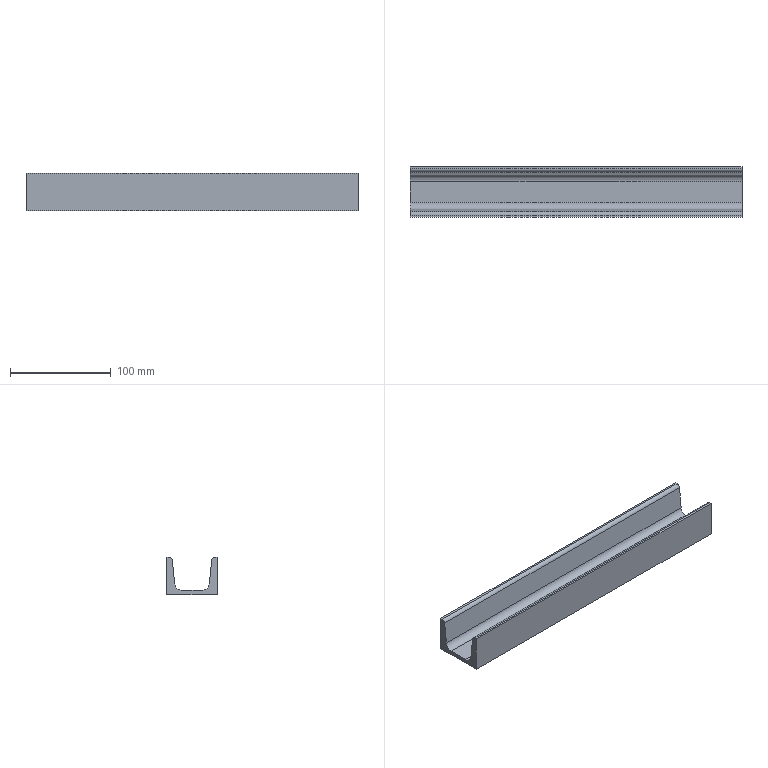Part | STEP file | HESS-408-70-15W-W-39-5# channel 1_default_machined_ | 1 solid | 14 faces | box 330 x 50 x 37 mm | volume 223683 mm3 | plane 10 | cylinder 4 | commonest cylinder face diameters 7 x2 14 x2
STEP:
#1=CARTESIAN_POINT('',(0.,0.,0.));
#2=DIRECTION('',(0.,0.,1.));
#3=DIRECTION('',(1.,0.,0.));
#4=AXIS2_PLACEMENT_3D('',#1,#2,#3);
#5=CARTESIAN_POINT('',(330.,0.,0.));
#6=VERTEX_POINT('',#5);
#7=CARTESIAN_POINT('',(0.,0.,0.));
#8=VERTEX_POINT('',#7);
#9=CARTESIAN_POINT('',(330.,0.,0.));
#10=DIRECTION('',(-1.,0.,0.));
#11=VECTOR('',#10,1.);
#12=LINE('',#9,#11);
#13=CARTESIAN_POINT('',(330.,0.,0.));
#14=DIRECTION('',(0.,0.,1.));
#15=DIRECTION('',(0.,-1.,0.));
#16=AXIS2_PLACEMENT_3D('',#13,#14,#15);
#17=PLANE('',#16);
#18=CARTESIAN_POINT('',(0.,0.));
#19=DIRECTION('',(0.,-1.));
#20=VECTOR('',#19,1.);
#21=LINE('',#18,#20);
#22=(GEOMETRIC_REPRESENTATION_CONTEXT(2)PARAMETRIC_REPRESENTATION_CONTEXT()REPRESENTATION_CONTEXT('',''));
#23=DEFINITIONAL_REPRESENTATION('',(#21),#22);
#24=PCURVE('',#17,#23);
#25=CARTESIAN_POINT('',(330.,0.,0.));
#26=DIRECTION('',(0.,-1.,0.));
#27=DIRECTION('',(0.,0.,-1.));
#28=AXIS2_PLACEMENT_3D('',#25,#26,#27);
#29=PLANE('',#28);
#30=CARTESIAN_POINT('',(0.,0.));
#31=DIRECTION('',(0.,-1.));
#32=VECTOR('',#31,1.);
#33=LINE('',#30,#32);
#34=(GEOMETRIC_REPRESENTATION_CONTEXT(2)PARAMETRIC_REPRESENTATION_CONTEXT()REPRESENTATION_CONTEXT('',''));
#35=DEFINITIONAL_REPRESENTATION('',(#33),#34);
#36=PCURVE('',#29,#35);
#37=SURFACE_CURVE('',#12,(#24,#36),.PCURVE_S1.);
#38=EDGE_CURVE('',#6,#8,#37,.T.);
#39=ORIENTED_EDGE('',*,*,#38,.F.);
#40=CARTESIAN_POINT('',(330.,-50.,0.));
#41=VERTEX_POINT('',#40);
#42=CARTESIAN_POINT('',(330.,0.,0.));
#43=DIRECTION('',(0.,1.,0.));
#44=VECTOR('',#43,1.);
#45=LINE('',#42,#44);
#46=CARTESIAN_POINT('',(0.,0.));
#47=DIRECTION('',(-1.,0.));
#48=VECTOR('',#47,1.);
#49=LINE('',#46,#48);
#50=(GEOMETRIC_REPRESENTATION_CONTEXT(2)PARAMETRIC_REPRESENTATION_CONTEXT()REPRESENTATION_CONTEXT('',''));
#51=DEFINITIONAL_REPRESENTATION('',(#49),#50);
#52=PCURVE('',#17,#51);
#53=CARTESIAN_POINT('',(330.,-48.017,33.5));
#54=DIRECTION('',(1.,0.,0.));
#55=DIRECTION('',(0.,1.,0.));
#56=AXIS2_PLACEMENT_3D('',#53,#54,#55);
#57=PLANE('',#56);
#58=CARTESIAN_POINT('',(48.017,-33.5));
#59=DIRECTION('',(1.,0.));
#60=VECTOR('',#59,1.);
#61=LINE('',#58,#60);
#62=(GEOMETRIC_REPRESENTATION_CONTEXT(2)PARAMETRIC_REPRESENTATION_CONTEXT()REPRESENTATION_CONTEXT('',''));
#63=DEFINITIONAL_REPRESENTATION('',(#61),#62);
#64=PCURVE('',#57,#63);
#65=SURFACE_CURVE('',#45,(#52,#64),.PCURVE_S1.);
#66=EDGE_CURVE('',#41,#6,#65,.T.);
#67=ORIENTED_EDGE('',*,*,#66,.F.);
#68=CARTESIAN_POINT('',(0.,-50.,0.));
#69=VERTEX_POINT('',#68);
#70=CARTESIAN_POINT('',(330.,-50.,0.));
#71=DIRECTION('',(1.,0.,0.));
#72=VECTOR('',#71,1.);
#73=LINE('',#70,#72);
#74=CARTESIAN_POINT('',(50.,0.));
#75=DIRECTION('',(0.,1.));
#76=VECTOR('',#75,1.);
#77=LINE('',#74,#76);
#78=(GEOMETRIC_REPRESENTATION_CONTEXT(2)PARAMETRIC_REPRESENTATION_CONTEXT()REPRESENTATION_CONTEXT('',''));
#79=DEFINITIONAL_REPRESENTATION('',(#77),#78);
#80=PCURVE('',#17,#79);
#81=CARTESIAN_POINT('',(330.,-50.,0.));
#82=DIRECTION('',(0.,1.,0.));
#83=DIRECTION('',(0.,0.,1.));
#84=AXIS2_PLACEMENT_3D('',#81,#82,#83);
#85=PLANE('',#84);
#86=CARTESIAN_POINT('',(0.,0.));
#87=DIRECTION('',(0.,1.));
#88=VECTOR('',#87,1.);
#89=LINE('',#86,#88);
#90=(GEOMETRIC_REPRESENTATION_CONTEXT(2)PARAMETRIC_REPRESENTATION_CONTEXT()REPRESENTATION_CONTEXT('',''));
#91=DEFINITIONAL_REPRESENTATION('',(#89),#90);
#92=PCURVE('',#85,#91);
#93=SURFACE_CURVE('',#73,(#80,#92),.PCURVE_S1.);
#94=EDGE_CURVE('',#69,#41,#93,.T.);
#95=ORIENTED_EDGE('',*,*,#94,.F.);
#96=CARTESIAN_POINT('',(0.,0.,0.));
#97=DIRECTION('',(0.,-1.,0.));
#98=VECTOR('',#97,1.);
#99=LINE('',#96,#98);
#100=CARTESIAN_POINT('',(0.,-330.));
#101=DIRECTION('',(1.,0.));
#102=VECTOR('',#101,1.);
#103=LINE('',#100,#102);
#104=(GEOMETRIC_REPRESENTATION_CONTEXT(2)PARAMETRIC_REPRESENTATION_CONTEXT()REPRESENTATION_CONTEXT('',''));
#105=DEFINITIONAL_REPRESENTATION('',(#103),#104);
#106=PCURVE('',#17,#105);
#107=CARTESIAN_POINT('',(0.,-48.017,33.5));
#108=DIRECTION('',(1.,0.,0.));
#109=DIRECTION('',(0.,1.,0.));
#110=AXIS2_PLACEMENT_3D('',#107,#108,#109);
#111=PLANE('',#110);
#112=CARTESIAN_POINT('',(48.017,-33.5));
#113=DIRECTION('',(-1.,0.));
#114=VECTOR('',#113,1.);
#115=LINE('',#112,#114);
#116=(GEOMETRIC_REPRESENTATION_CONTEXT(2)PARAMETRIC_REPRESENTATION_CONTEXT()REPRESENTATION_CONTEXT('',''));
#117=DEFINITIONAL_REPRESENTATION('',(#115),#116);
#118=PCURVE('',#111,#117);
#119=SURFACE_CURVE('',#99,(#106,#118),.PCURVE_S1.);
#120=EDGE_CURVE('',#8,#69,#119,.T.);
#121=ORIENTED_EDGE('',*,*,#120,.F.);
#122=EDGE_LOOP('',(#39,#67,#95,#121));
#123=FACE_BOUND('',#122,.T.);
#124=ADVANCED_FACE('',(#123),#17,.F.);
#125=CARTESIAN_POINT('',(0.,-48.017,37.));
#126=VERTEX_POINT('',#125);
#127=CARTESIAN_POINT('',(0.,-50.,37.));
#128=VERTEX_POINT('',#127);
#129=CARTESIAN_POINT('',(0.,-48.017,37.));
#130=DIRECTION('',(0.,-1.,0.));
#131=VECTOR('',#130,1.);
#132=LINE('',#129,#131);
#133=CARTESIAN_POINT('',(0.,3.5));
#134=DIRECTION('',(-1.,0.));
#135=VECTOR('',#134,1.);
#136=LINE('',#133,#135);
#137=(GEOMETRIC_REPRESENTATION_CONTEXT(2)PARAMETRIC_REPRESENTATION_CONTEXT()REPRESENTATION_CONTEXT('',''));
#138=DEFINITIONAL_REPRESENTATION('',(#136),#137);
#139=PCURVE('',#111,#138);
#140=CARTESIAN_POINT('',(330.,-48.017,37.));
#141=DIRECTION('',(0.,0.,-1.));
#142=DIRECTION('',(0.,1.,0.));
#143=AXIS2_PLACEMENT_3D('',#140,#141,#142);
#144=PLANE('',#143);
#145=CARTESIAN_POINT('',(0.,-330.));
#146=DIRECTION('',(-1.,0.));
#147=VECTOR('',#146,1.);
#148=LINE('',#145,#147);
#149=(GEOMETRIC_REPRESENTATION_CONTEXT(2)PARAMETRIC_REPRESENTATION_CONTEXT()REPRESENTATION_CONTEXT('',''));
#150=DEFINITIONAL_REPRESENTATION('',(#148),#149);
#151=PCURVE('',#144,#150);
#152=SURFACE_CURVE('',#132,(#139,#151),.PCURVE_S1.);
#153=EDGE_CURVE('',#126,#128,#152,.T.);
#154=ORIENTED_EDGE('',*,*,#153,.F.);
#155=CARTESIAN_POINT('',(0.,-44.535,33.848));
#156=VERTEX_POINT('',#155);
#157=CARTESIAN_POINT('',(0.,-48.017,33.5));
#158=DIRECTION('',(1.,0.,0.));
#159=DIRECTION('',(0.,-1.,0.));
#160=AXIS2_PLACEMENT_3D('',#157,#158,#159);
#161=CIRCLE('',#160,3.5);
#162=CARTESIAN_POINT('',(0.,0.));
#163=DIRECTION('',(-1.,0.));
#164=AXIS2_PLACEMENT_2D('',#162,#163);
#165=CIRCLE('',#164,3.5);
#166=(GEOMETRIC_REPRESENTATION_CONTEXT(2)PARAMETRIC_REPRESENTATION_CONTEXT()REPRESENTATION_CONTEXT('',''));
#167=DEFINITIONAL_REPRESENTATION('',(#165),#166);
#168=PCURVE('',#111,#167);
#169=CARTESIAN_POINT('',(330.,-48.017,33.5));
#170=DIRECTION('',(-1.,0.,0.));
#171=DIRECTION('',(0.,-1.,0.));
#172=AXIS2_PLACEMENT_3D('',#169,#170,#171);
#173=CYLINDRICAL_SURFACE('',#172,3.5);
#174=CARTESIAN_POINT('',(6.283,330.));
#175=DIRECTION('',(-1.,0.));
#176=VECTOR('',#175,1.);
#177=LINE('',#174,#176);
#178=(GEOMETRIC_REPRESENTATION_CONTEXT(2)PARAMETRIC_REPRESENTATION_CONTEXT()REPRESENTATION_CONTEXT('',''));
#179=DEFINITIONAL_REPRESENTATION('',(#177),#178);
#180=PCURVE('',#173,#179);
#181=SURFACE_CURVE('',#161,(#168,#180),.PCURVE_S1.);
#182=EDGE_CURVE('',#156,#126,#181,.T.);
#183=ORIENTED_EDGE('',*,*,#182,.F.);
#184=CARTESIAN_POINT('',(0.,-42.23,10.803));
#185=VERTEX_POINT('',#184);
#186=CARTESIAN_POINT('',(0.,-42.23,10.803));
#187=DIRECTION('',(0.,-0.0995,0.995));
#188=VECTOR('',#187,1.);
#189=LINE('',#186,#188);
#190=CARTESIAN_POINT('',(5.787,-22.697));
#191=DIRECTION('',(-0.0995,0.995));
#192=VECTOR('',#191,1.);
#193=LINE('',#190,#192);
#194=(GEOMETRIC_REPRESENTATION_CONTEXT(2)PARAMETRIC_REPRESENTATION_CONTEXT()REPRESENTATION_CONTEXT('',''));
#195=DEFINITIONAL_REPRESENTATION('',(#193),#194);
#196=PCURVE('',#111,#195);
#197=CARTESIAN_POINT('',(330.,-42.23,10.803));
#198=DIRECTION('',(0.,-0.995,-0.0995));
#199=DIRECTION('',(0.,0.0995,-0.995));
#200=AXIS2_PLACEMENT_3D('',#197,#198,#199);
#201=PLANE('',#200);
#202=CARTESIAN_POINT('',(0.,-330.));
#203=DIRECTION('',(-1.,0.));
#204=VECTOR('',#203,1.);
#205=LINE('',#202,#204);
#206=(GEOMETRIC_REPRESENTATION_CONTEXT(2)PARAMETRIC_REPRESENTATION_CONTEXT()REPRESENTATION_CONTEXT('',''));
#207=DEFINITIONAL_REPRESENTATION('',(#205),#206);
#208=PCURVE('',#201,#207);
#209=SURFACE_CURVE('',#189,(#196,#208),.PCURVE_S1.);
#210=EDGE_CURVE('',#185,#156,#209,.T.);
#211=ORIENTED_EDGE('',*,*,#210,.F.);
#212=CARTESIAN_POINT('',(0.,-35.265,4.5));
#213=VERTEX_POINT('',#212);
#214=CARTESIAN_POINT('',(0.,-35.265,11.5));
#215=DIRECTION('',(-1.,0.,0.));
#216=DIRECTION('',(0.,-1.,0.));
#217=AXIS2_PLACEMENT_3D('',#214,#215,#216);
#218=CIRCLE('',#217,7.);
#219=CARTESIAN_POINT('',(5.752,-22.));
#220=CARTESIAN_POINT('',(5.752,-9.876));
#221=CARTESIAN_POINT('',(16.252,-15.938));
#222=CARTESIAN_POINT('',(26.752,-22.));
#223=CARTESIAN_POINT('',(16.252,-28.062));
#224=CARTESIAN_POINT('',(5.752,-34.124));
#225=CARTESIAN_POINT('',(5.752,-22.));
#226=(BOUNDED_CURVE()B_SPLINE_CURVE(2,(#219,#220,#221,#222,#223,#224,#225),.UNSPECIFIED.,.T.,.F.)B_SPLINE_CURVE_WITH_KNOTS((1,2,2,2,2,1),(-2.094,0.,2.094,4.189,6.283,8.378),.UNSPECIFIED.)CURVE()GEOMETRIC_REPRESENTATION_ITEM()RATIONAL_B_SPLINE_CURVE((1.,0.5,1.,0.5,1.,0.5,1.))REPRESENTATION_ITEM(''));
#227=(GEOMETRIC_REPRESENTATION_CONTEXT(2)PARAMETRIC_REPRESENTATION_CONTEXT()REPRESENTATION_CONTEXT('',''));
#228=DEFINITIONAL_REPRESENTATION('',(#226),#227);
#229=PCURVE('',#111,#228);
#230=CARTESIAN_POINT('',(330.,-35.265,11.5));
#231=DIRECTION('',(-1.,0.,0.));
#232=DIRECTION('',(0.,-1.,0.));
#233=AXIS2_PLACEMENT_3D('',#230,#231,#232);
#234=CYLINDRICAL_SURFACE('',#233,7.);
#235=CARTESIAN_POINT('',(0.,330.));
#236=DIRECTION('',(1.,0.));
#237=VECTOR('',#236,1.);
#238=LINE('',#235,#237);
#239=(GEOMETRIC_REPRESENTATION_CONTEXT(2)PARAMETRIC_REPRESENTATION_CONTEXT()REPRESENTATION_CONTEXT('',''));
#240=DEFINITIONAL_REPRESENTATION('',(#238),#239);
#241=PCURVE('',#234,#240);
#242=SURFACE_CURVE('',#218,(#229,#241),.PCURVE_S1.);
#243=EDGE_CURVE('',#213,#185,#242,.T.);
#244=ORIENTED_EDGE('',*,*,#243,.F.);
#245=CARTESIAN_POINT('',(0.,-14.735,4.5));
#246=VERTEX_POINT('',#245);
#247=CARTESIAN_POINT('',(0.,-48.017,4.5));
#248=DIRECTION('',(0.,-1.,0.));
#249=VECTOR('',#248,1.);
#250=LINE('',#247,#249);
#251=CARTESIAN_POINT('',(0.,-29.));
#252=DIRECTION('',(-1.,0.));
#253=VECTOR('',#252,1.);
#254=LINE('',#251,#253);
#255=(GEOMETRIC_REPRESENTATION_CONTEXT(2)PARAMETRIC_REPRESENTATION_CONTEXT()REPRESENTATION_CONTEXT('',''));
#256=DEFINITIONAL_REPRESENTATION('',(#254),#255);
#257=PCURVE('',#111,#256);
#258=CARTESIAN_POINT('',(330.,-35.265,4.5));
#259=DIRECTION('',(0.,0.,-1.));
#260=DIRECTION('',(0.,1.,0.));
#261=AXIS2_PLACEMENT_3D('',#258,#259,#260);
#262=PLANE('',#261);
#263=CARTESIAN_POINT('',(-12.752,-330.));
#264=DIRECTION('',(-1.,0.));
#265=VECTOR('',#264,1.);
#266=LINE('',#263,#265);
#267=(GEOMETRIC_REPRESENTATION_CONTEXT(2)PARAMETRIC_REPRESENTATION_CONTEXT()REPRESENTATION_CONTEXT('',''));
#268=DEFINITIONAL_REPRESENTATION('',(#266),#267);
#269=PCURVE('',#262,#268);
#270=SURFACE_CURVE('',#250,(#257,#269),.PCURVE_S1.);
#271=EDGE_CURVE('',#246,#213,#270,.T.);
#272=ORIENTED_EDGE('',*,*,#271,.F.);
#273=CARTESIAN_POINT('',(0.,-7.77,10.803));
#274=VERTEX_POINT('',#273);
#275=CARTESIAN_POINT('',(0.,-14.735,11.5));
#276=DIRECTION('',(-1.,0.,0.));
#277=DIRECTION('',(0.,-1.,0.));
#278=AXIS2_PLACEMENT_3D('',#275,#276,#277);
#279=CIRCLE('',#278,7.);
#280=CARTESIAN_POINT('',(26.283,-22.));
#281=CARTESIAN_POINT('',(26.283,-9.876));
#282=CARTESIAN_POINT('',(36.783,-15.938));
#283=CARTESIAN_POINT('',(47.283,-22.));
#284=CARTESIAN_POINT('',(36.783,-28.062));
#285=CARTESIAN_POINT('',(26.283,-34.124));
#286=CARTESIAN_POINT('',(26.283,-22.));
#287=(BOUNDED_CURVE()B_SPLINE_CURVE(2,(#280,#281,#282,#283,#284,#285,#286),.UNSPECIFIED.,.T.,.F.)B_SPLINE_CURVE_WITH_KNOTS((1,2,2,2,2,1),(-2.094,0.,2.094,4.189,6.283,8.378),.UNSPECIFIED.)CURVE()GEOMETRIC_REPRESENTATION_ITEM()RATIONAL_B_SPLINE_CURVE((1.,0.5,1.,0.5,1.,0.5,1.))REPRESENTATION_ITEM(''));
#288=(GEOMETRIC_REPRESENTATION_CONTEXT(2)PARAMETRIC_REPRESENTATION_CONTEXT()REPRESENTATION_CONTEXT('',''));
#289=DEFINITIONAL_REPRESENTATION('',(#287),#288);
#290=PCURVE('',#111,#289);
#291=CARTESIAN_POINT('',(330.,-14.735,11.5));
#292=DIRECTION('',(-1.,0.,0.));
#293=DIRECTION('',(0.,-1.,0.));
#294=AXIS2_PLACEMENT_3D('',#291,#292,#293);
#295=CYLINDRICAL_SURFACE('',#294,7.);
#296=CARTESIAN_POINT('',(0.,330.));
#297=DIRECTION('',(1.,0.));
#298=VECTOR('',#297,1.);
#299=LINE('',#296,#298);
#300=(GEOMETRIC_REPRESENTATION_CONTEXT(2)PARAMETRIC_REPRESENTATION_CONTEXT()REPRESENTATION_CONTEXT('',''));
#301=DEFINITIONAL_REPRESENTATION('',(#299),#300);
#302=PCURVE('',#295,#301);
#303=SURFACE_CURVE('',#279,(#290,#302),.PCURVE_S1.);
#304=EDGE_CURVE('',#274,#246,#303,.T.);
#305=ORIENTED_EDGE('',*,*,#304,.F.);
#306=CARTESIAN_POINT('',(0.,-5.465,33.848));
#307=VERTEX_POINT('',#306);
#308=CARTESIAN_POINT('',(0.,-5.465,33.848));
#309=DIRECTION('',(0.,-0.0995,-0.995));
#310=VECTOR('',#309,1.);
#311=LINE('',#308,#310);
#312=CARTESIAN_POINT('',(42.552,0.3483));
#313=DIRECTION('',(-0.0995,-0.995));
#314=VECTOR('',#313,1.);
#315=LINE('',#312,#314);
#316=(GEOMETRIC_REPRESENTATION_CONTEXT(2)PARAMETRIC_REPRESENTATION_CONTEXT()REPRESENTATION_CONTEXT('',''));
#317=DEFINITIONAL_REPRESENTATION('',(#315),#316);
#318=PCURVE('',#111,#317);
#319=CARTESIAN_POINT('',(330.,-7.77,10.803));
#320=DIRECTION('',(0.,0.995,-0.0995));
#321=DIRECTION('',(0.,0.0995,0.995));
#322=AXIS2_PLACEMENT_3D('',#319,#320,#321);
#323=PLANE('',#322);
#324=CARTESIAN_POINT('',(23.16,-330.));
#325=DIRECTION('',(-1.,0.));
#326=VECTOR('',#325,1.);
#327=LINE('',#324,#326);
#328=(GEOMETRIC_REPRESENTATION_CONTEXT(2)PARAMETRIC_REPRESENTATION_CONTEXT()REPRESENTATION_CONTEXT('',''));
#329=DEFINITIONAL_REPRESENTATION('',(#327),#328);
#330=PCURVE('',#323,#329);
#331=SURFACE_CURVE('',#311,(#318,#330),.PCURVE_S1.);
#332=EDGE_CURVE('',#307,#274,#331,.T.);
#333=ORIENTED_EDGE('',*,*,#332,.F.);
#334=CARTESIAN_POINT('',(0.,-1.983,37.));
#335=VERTEX_POINT('',#334);
#336=CARTESIAN_POINT('',(0.,-1.983,33.5));
#337=DIRECTION('',(1.,0.,0.));
#338=DIRECTION('',(0.,-1.,0.));
#339=AXIS2_PLACEMENT_3D('',#336,#337,#338);
#340=CIRCLE('',#339,3.5);
#341=CARTESIAN_POINT('',(46.035,0.));
#342=DIRECTION('',(-1.,0.));
#343=AXIS2_PLACEMENT_2D('',#341,#342);
#344=CIRCLE('',#343,3.5);
#345=(GEOMETRIC_REPRESENTATION_CONTEXT(2)PARAMETRIC_REPRESENTATION_CONTEXT()REPRESENTATION_CONTEXT('',''));
#346=DEFINITIONAL_REPRESENTATION('',(#344),#345);
#347=PCURVE('',#111,#346);
#348=CARTESIAN_POINT('',(330.,-1.983,33.5));
#349=DIRECTION('',(-1.,0.,0.));
#350=DIRECTION('',(0.,-1.,0.));
#351=AXIS2_PLACEMENT_3D('',#348,#349,#350);
#352=CYLINDRICAL_SURFACE('',#351,3.5);
#353=CARTESIAN_POINT('',(6.283,330.));
#354=DIRECTION('',(-1.,0.));
#355=VECTOR('',#354,1.);
#356=LINE('',#353,#355);
#357=(GEOMETRIC_REPRESENTATION_CONTEXT(2)PARAMETRIC_REPRESENTATION_CONTEXT()REPRESENTATION_CONTEXT('',''));
#358=DEFINITIONAL_REPRESENTATION('',(#356),#357);
#359=PCURVE('',#352,#358);
#360=SURFACE_CURVE('',#340,(#347,#359),.PCURVE_S1.);
#361=EDGE_CURVE('',#335,#307,#360,.T.);
#362=ORIENTED_EDGE('',*,*,#361,.F.);
#363=CARTESIAN_POINT('',(0.,0.,37.));
#364=VERTEX_POINT('',#363);
#365=CARTESIAN_POINT('',(0.,-48.017,37.));
#366=DIRECTION('',(0.,-1.,0.));
#367=VECTOR('',#366,1.);
#368=LINE('',#365,#367);
#369=CARTESIAN_POINT('',(0.,3.5));
#370=DIRECTION('',(-1.,0.));
#371=VECTOR('',#370,1.);
#372=LINE('',#369,#371);
#373=(GEOMETRIC_REPRESENTATION_CONTEXT(2)PARAMETRIC_REPRESENTATION_CONTEXT()REPRESENTATION_CONTEXT('',''));
#374=DEFINITIONAL_REPRESENTATION('',(#372),#373);
#375=PCURVE('',#111,#374);
#376=CARTESIAN_POINT('',(330.,-1.983,37.));
#377=DIRECTION('',(0.,0.,-1.));
#378=DIRECTION('',(0.,1.,0.));
#379=AXIS2_PLACEMENT_3D('',#376,#377,#378);
#380=PLANE('',#379);
#381=CARTESIAN_POINT('',(-46.035,-330.));
#382=DIRECTION('',(-1.,0.));
#383=VECTOR('',#382,1.);
#384=LINE('',#381,#383);
#385=(GEOMETRIC_REPRESENTATION_CONTEXT(2)PARAMETRIC_REPRESENTATION_CONTEXT()REPRESENTATION_CONTEXT('',''));
#386=DEFINITIONAL_REPRESENTATION('',(#384),#385);
#387=PCURVE('',#380,#386);
#388=SURFACE_CURVE('',#368,(#375,#387),.PCURVE_S1.);
#389=EDGE_CURVE('',#364,#335,#388,.T.);
#390=ORIENTED_EDGE('',*,*,#389,.F.);
#391=CARTESIAN_POINT('',(0.,0.,33.5));
#392=DIRECTION('',(0.,0.,1.));
#393=VECTOR('',#392,1.);
#394=LINE('',#391,#393);
#395=CARTESIAN_POINT('',(48.017,0.));
#396=DIRECTION('',(0.,1.));
#397=VECTOR('',#396,1.);
#398=LINE('',#395,#397);
#399=(GEOMETRIC_REPRESENTATION_CONTEXT(2)PARAMETRIC_REPRESENTATION_CONTEXT()REPRESENTATION_CONTEXT('',''));
#400=DEFINITIONAL_REPRESENTATION('',(#398),#399);
#401=PCURVE('',#111,#400);
#402=CARTESIAN_POINT('',(-33.5,-330.));
#403=DIRECTION('',(-1.,0.));
#404=VECTOR('',#403,1.);
#405=LINE('',#402,#404);
#406=(GEOMETRIC_REPRESENTATION_CONTEXT(2)PARAMETRIC_REPRESENTATION_CONTEXT()REPRESENTATION_CONTEXT('',''));
#407=DEFINITIONAL_REPRESENTATION('',(#405),#406);
#408=PCURVE('',#29,#407);
#409=SURFACE_CURVE('',#394,(#401,#408),.PCURVE_S1.);
#410=EDGE_CURVE('',#8,#364,#409,.T.);
#411=ORIENTED_EDGE('',*,*,#410,.F.);
#412=ORIENTED_EDGE('',*,*,#120,.T.);
#413=CARTESIAN_POINT('',(0.,-50.,33.5));
#414=DIRECTION('',(0.,0.,-1.));
#415=VECTOR('',#414,1.);
#416=LINE('',#413,#415);
#417=CARTESIAN_POINT('',(-1.983,0.));
#418=DIRECTION('',(0.,-1.));
#419=VECTOR('',#418,1.);
#420=LINE('',#417,#419);
#421=(GEOMETRIC_REPRESENTATION_CONTEXT(2)PARAMETRIC_REPRESENTATION_CONTEXT()REPRESENTATION_CONTEXT('',''));
#422=DEFINITIONAL_REPRESENTATION('',(#420),#421);
#423=PCURVE('',#111,#422);
#424=CARTESIAN_POINT('',(33.5,-330.));
#425=DIRECTION('',(-1.,0.));
#426=VECTOR('',#425,1.);
#427=LINE('',#424,#426);
#428=(GEOMETRIC_REPRESENTATION_CONTEXT(2)PARAMETRIC_REPRESENTATION_CONTEXT()REPRESENTATION_CONTEXT('',''));
#429=DEFINITIONAL_REPRESENTATION('',(#427),#428);
#430=PCURVE('',#85,#429);
#431=SURFACE_CURVE('',#416,(#423,#430),.PCURVE_S1.);
#432=EDGE_CURVE('',#128,#69,#431,.T.);
#433=ORIENTED_EDGE('',*,*,#432,.F.);
#434=EDGE_LOOP('',(#154,#183,#211,#244,#272,#305,#333,#362,#390,#411,#412,#433));
#435=FACE_BOUND('',#434,.T.);
#436=ADVANCED_FACE('',(#435),#111,.F.);
#437=CARTESIAN_POINT('',(330.,0.,37.));
#438=VERTEX_POINT('',#437);
#439=CARTESIAN_POINT('',(330.,0.,37.));
#440=DIRECTION('',(-1.,0.,0.));
#441=VECTOR('',#440,1.);
#442=LINE('',#439,#441);
#443=CARTESIAN_POINT('',(-37.,0.));
#444=DIRECTION('',(0.,-1.));
#445=VECTOR('',#444,1.);
#446=LINE('',#443,#445);
#447=(GEOMETRIC_REPRESENTATION_CONTEXT(2)PARAMETRIC_REPRESENTATION_CONTEXT()REPRESENTATION_CONTEXT('',''));
#448=DEFINITIONAL_REPRESENTATION('',(#446),#447);
#449=PCURVE('',#29,#448);
#450=CARTESIAN_POINT('',(1.983,0.));
#451=DIRECTION('',(0.,-1.));
#452=VECTOR('',#451,1.);
#453=LINE('',#450,#452);
#454=(GEOMETRIC_REPRESENTATION_CONTEXT(2)PARAMETRIC_REPRESENTATION_CONTEXT()REPRESENTATION_CONTEXT('',''));
#455=DEFINITIONAL_REPRESENTATION('',(#453),#454);
#456=PCURVE('',#380,#455);
#457=SURFACE_CURVE('',#442,(#449,#456),.PCURVE_S1.);
#458=EDGE_CURVE('',#438,#364,#457,.T.);
#459=ORIENTED_EDGE('',*,*,#458,.F.);
#460=CARTESIAN_POINT('',(330.,0.,0.));
#461=DIRECTION('',(0.,0.,1.));
#462=VECTOR('',#461,1.);
#463=LINE('',#460,#462);
#464=CARTESIAN_POINT('',(0.,0.));
#465=DIRECTION('',(-1.,0.));
#466=VECTOR('',#465,1.);
#467=LINE('',#464,#466);
#468=(GEOMETRIC_REPRESENTATION_CONTEXT(2)PARAMETRIC_REPRESENTATION_CONTEXT()REPRESENTATION_CONTEXT('',''));
#469=DEFINITIONAL_REPRESENTATION('',(#467),#468);
#470=PCURVE('',#29,#469);
#471=CARTESIAN_POINT('',(48.017,-33.5));
#472=DIRECTION('',(0.,1.));
#473=VECTOR('',#472,1.);
#474=LINE('',#471,#473);
#475=(GEOMETRIC_REPRESENTATION_CONTEXT(2)PARAMETRIC_REPRESENTATION_CONTEXT()REPRESENTATION_CONTEXT('',''));
#476=DEFINITIONAL_REPRESENTATION('',(#474),#475);
#477=PCURVE('',#57,#476);
#478=SURFACE_CURVE('',#463,(#470,#477),.PCURVE_S1.);
#479=EDGE_CURVE('',#6,#438,#478,.T.);
#480=ORIENTED_EDGE('',*,*,#479,.F.);
#481=ORIENTED_EDGE('',*,*,#38,.T.);
#482=ORIENTED_EDGE('',*,*,#410,.T.);
#483=EDGE_LOOP('',(#459,#480,#481,#482));
#484=FACE_BOUND('',#483,.T.);
#485=ADVANCED_FACE('',(#484),#29,.F.);
#486=CARTESIAN_POINT('',(330.,-44.535,33.848));
#487=VERTEX_POINT('',#486);
#488=CARTESIAN_POINT('',(330.,-48.017,37.));
#489=VERTEX_POINT('',#488);
#490=CARTESIAN_POINT('',(330.,-48.017,33.5));
#491=DIRECTION('',(1.,0.,0.));
#492=DIRECTION('',(0.,-1.,0.));
#493=AXIS2_PLACEMENT_3D('',#490,#491,#492);
#494=CIRCLE('',#493,3.5);
#495=CARTESIAN_POINT('',(0.,0.));
#496=DIRECTION('',(-1.,0.));
#497=AXIS2_PLACEMENT_2D('',#495,#496);
#498=CIRCLE('',#497,3.5);
#499=(GEOMETRIC_REPRESENTATION_CONTEXT(2)PARAMETRIC_REPRESENTATION_CONTEXT()REPRESENTATION_CONTEXT('',''));
#500=DEFINITIONAL_REPRESENTATION('',(#498),#499);
#501=PCURVE('',#57,#500);
#502=CARTESIAN_POINT('',(6.283,0.));
#503=DIRECTION('',(-1.,0.));
#504=VECTOR('',#503,1.);
#505=LINE('',#502,#504);
#506=(GEOMETRIC_REPRESENTATION_CONTEXT(2)PARAMETRIC_REPRESENTATION_CONTEXT()REPRESENTATION_CONTEXT('',''));
#507=DEFINITIONAL_REPRESENTATION('',(#505),#506);
#508=PCURVE('',#173,#507);
#509=SURFACE_CURVE('',#494,(#501,#508),.PCURVE_S1.);
#510=EDGE_CURVE('',#487,#489,#509,.T.);
#511=ORIENTED_EDGE('',*,*,#510,.T.);
#512=CARTESIAN_POINT('',(330.,-50.,37.));
#513=VERTEX_POINT('',#512);
#514=CARTESIAN_POINT('',(330.,-48.017,37.));
#515=DIRECTION('',(0.,-1.,0.));
#516=VECTOR('',#515,1.);
#517=LINE('',#514,#516);
#518=CARTESIAN_POINT('',(0.,3.5));
#519=DIRECTION('',(-1.,0.));
#520=VECTOR('',#519,1.);
#521=LINE('',#518,#520);
#522=(GEOMETRIC_REPRESENTATION_CONTEXT(2)PARAMETRIC_REPRESENTATION_CONTEXT()REPRESENTATION_CONTEXT('',''));
#523=DEFINITIONAL_REPRESENTATION('',(#521),#522);
#524=PCURVE('',#57,#523);
#525=CARTESIAN_POINT('',(0.,0.));
#526=DIRECTION('',(-1.,0.));
#527=VECTOR('',#526,1.);
#528=LINE('',#525,#527);
#529=(GEOMETRIC_REPRESENTATION_CONTEXT(2)PARAMETRIC_REPRESENTATION_CONTEXT()REPRESENTATION_CONTEXT('',''));
#530=DEFINITIONAL_REPRESENTATION('',(#528),#529);
#531=PCURVE('',#144,#530);
#532=SURFACE_CURVE('',#517,(#524,#531),.PCURVE_S1.);
#533=EDGE_CURVE('',#489,#513,#532,.T.);
#534=ORIENTED_EDGE('',*,*,#533,.T.);
#535=CARTESIAN_POINT('',(330.,-50.,33.5));
#536=DIRECTION('',(0.,0.,-1.));
#537=VECTOR('',#536,1.);
#538=LINE('',#535,#537);
#539=CARTESIAN_POINT('',(-1.983,0.));
#540=DIRECTION('',(0.,-1.));
#541=VECTOR('',#540,1.);
#542=LINE('',#539,#541);
#543=(GEOMETRIC_REPRESENTATION_CONTEXT(2)PARAMETRIC_REPRESENTATION_CONTEXT()REPRESENTATION_CONTEXT('',''));
#544=DEFINITIONAL_REPRESENTATION('',(#542),#543);
#545=PCURVE('',#57,#544);
#546=CARTESIAN_POINT('',(33.5,0.));
#547=DIRECTION('',(-1.,0.));
#548=VECTOR('',#547,1.);
#549=LINE('',#546,#548);
#550=(GEOMETRIC_REPRESENTATION_CONTEXT(2)PARAMETRIC_REPRESENTATION_CONTEXT()REPRESENTATION_CONTEXT('',''));
#551=DEFINITIONAL_REPRESENTATION('',(#549),#550);
#552=PCURVE('',#85,#551);
#553=SURFACE_CURVE('',#538,(#545,#552),.PCURVE_S1.);
#554=EDGE_CURVE('',#513,#41,#553,.T.);
#555=ORIENTED_EDGE('',*,*,#554,.T.);
#556=ORIENTED_EDGE('',*,*,#66,.T.);
#557=ORIENTED_EDGE('',*,*,#479,.T.);
#558=CARTESIAN_POINT('',(330.,-1.983,37.));
#559=VERTEX_POINT('',#558);
#560=CARTESIAN_POINT('',(330.,-48.017,37.));
#561=DIRECTION('',(0.,-1.,0.));
#562=VECTOR('',#561,1.);
#563=LINE('',#560,#562);
#564=CARTESIAN_POINT('',(0.,3.5));
#565=DIRECTION('',(-1.,0.));
#566=VECTOR('',#565,1.);
#567=LINE('',#564,#566);
#568=(GEOMETRIC_REPRESENTATION_CONTEXT(2)PARAMETRIC_REPRESENTATION_CONTEXT()REPRESENTATION_CONTEXT('',''));
#569=DEFINITIONAL_REPRESENTATION('',(#567),#568);
#570=PCURVE('',#57,#569);
#571=CARTESIAN_POINT('',(-46.035,0.));
#572=DIRECTION('',(-1.,0.));
#573=VECTOR('',#572,1.);
#574=LINE('',#571,#573);
#575=(GEOMETRIC_REPRESENTATION_CONTEXT(2)PARAMETRIC_REPRESENTATION_CONTEXT()REPRESENTATION_CONTEXT('',''));
#576=DEFINITIONAL_REPRESENTATION('',(#574),#575);
#577=PCURVE('',#380,#576);
#578=SURFACE_CURVE('',#563,(#570,#577),.PCURVE_S1.);
#579=EDGE_CURVE('',#438,#559,#578,.T.);
#580=ORIENTED_EDGE('',*,*,#579,.T.);
#581=CARTESIAN_POINT('',(330.,-5.465,33.848));
#582=VERTEX_POINT('',#581);
#583=CARTESIAN_POINT('',(330.,-1.983,33.5));
#584=DIRECTION('',(1.,0.,0.));
#585=DIRECTION('',(0.,-1.,0.));
#586=AXIS2_PLACEMENT_3D('',#583,#584,#585);
#587=CIRCLE('',#586,3.5);
#588=CARTESIAN_POINT('',(46.035,0.));
#589=DIRECTION('',(-1.,0.));
#590=AXIS2_PLACEMENT_2D('',#588,#589);
#591=CIRCLE('',#590,3.5);
#592=(GEOMETRIC_REPRESENTATION_CONTEXT(2)PARAMETRIC_REPRESENTATION_CONTEXT()REPRESENTATION_CONTEXT('',''));
#593=DEFINITIONAL_REPRESENTATION('',(#591),#592);
#594=PCURVE('',#57,#593);
#595=CARTESIAN_POINT('',(6.283,0.));
#596=DIRECTION('',(-1.,0.));
#597=VECTOR('',#596,1.);
#598=LINE('',#595,#597);
#599=(GEOMETRIC_REPRESENTATION_CONTEXT(2)PARAMETRIC_REPRESENTATION_CONTEXT()REPRESENTATION_CONTEXT('',''));
#600=DEFINITIONAL_REPRESENTATION('',(#598),#599);
#601=PCURVE('',#352,#600);
#602=SURFACE_CURVE('',#587,(#594,#601),.PCURVE_S1.);
#603=EDGE_CURVE('',#559,#582,#602,.T.);
#604=ORIENTED_EDGE('',*,*,#603,.T.);
#605=CARTESIAN_POINT('',(330.,-7.77,10.803));
#606=VERTEX_POINT('',#605);
#607=CARTESIAN_POINT('',(330.,-5.465,33.848));
#608=DIRECTION('',(0.,-0.0995,-0.995));
#609=VECTOR('',#608,1.);
#610=LINE('',#607,#609);
#611=CARTESIAN_POINT('',(42.552,0.3483));
#612=DIRECTION('',(-0.0995,-0.995));
#613=VECTOR('',#612,1.);
#614=LINE('',#611,#613);
#615=(GEOMETRIC_REPRESENTATION_CONTEXT(2)PARAMETRIC_REPRESENTATION_CONTEXT()REPRESENTATION_CONTEXT('',''));
#616=DEFINITIONAL_REPRESENTATION('',(#614),#615);
#617=PCURVE('',#57,#616);
#618=CARTESIAN_POINT('',(23.16,0.));
#619=DIRECTION('',(-1.,0.));
#620=VECTOR('',#619,1.);
#621=LINE('',#618,#620);
#622=(GEOMETRIC_REPRESENTATION_CONTEXT(2)PARAMETRIC_REPRESENTATION_CONTEXT()REPRESENTATION_CONTEXT('',''));
#623=DEFINITIONAL_REPRESENTATION('',(#621),#622);
#624=PCURVE('',#323,#623);
#625=SURFACE_CURVE('',#610,(#617,#624),.PCURVE_S1.);
#626=EDGE_CURVE('',#582,#606,#625,.T.);
#627=ORIENTED_EDGE('',*,*,#626,.T.);
#628=CARTESIAN_POINT('',(330.,-14.735,4.5));
#629=VERTEX_POINT('',#628);
#630=CARTESIAN_POINT('',(330.,-14.735,11.5));
#631=DIRECTION('',(-1.,0.,0.));
#632=DIRECTION('',(0.,-1.,0.));
#633=AXIS2_PLACEMENT_3D('',#630,#631,#632);
#634=CIRCLE('',#633,7.);
#635=CARTESIAN_POINT('',(26.283,-22.));
#636=CARTESIAN_POINT('',(26.283,-9.876));
#637=CARTESIAN_POINT('',(36.783,-15.938));
#638=CARTESIAN_POINT('',(47.283,-22.));
#639=CARTESIAN_POINT('',(36.783,-28.062));
#640=CARTESIAN_POINT('',(26.283,-34.124));
#641=CARTESIAN_POINT('',(26.283,-22.));
#642=(BOUNDED_CURVE()B_SPLINE_CURVE(2,(#635,#636,#637,#638,#639,#640,#641),.UNSPECIFIED.,.T.,.F.)B_SPLINE_CURVE_WITH_KNOTS((1,2,2,2,2,1),(-2.094,0.,2.094,4.189,6.283,8.378),.UNSPECIFIED.)CURVE()GEOMETRIC_REPRESENTATION_ITEM()RATIONAL_B_SPLINE_CURVE((1.,0.5,1.,0.5,1.,0.5,1.))REPRESENTATION_ITEM(''));
#643=(GEOMETRIC_REPRESENTATION_CONTEXT(2)PARAMETRIC_REPRESENTATION_CONTEXT()REPRESENTATION_CONTEXT('',''));
#644=DEFINITIONAL_REPRESENTATION('',(#642),#643);
#645=PCURVE('',#57,#644);
#646=CARTESIAN_POINT('',(0.,0.));
#647=DIRECTION('',(1.,0.));
#648=VECTOR('',#647,1.);
#649=LINE('',#646,#648);
#650=(GEOMETRIC_REPRESENTATION_CONTEXT(2)PARAMETRIC_REPRESENTATION_CONTEXT()REPRESENTATION_CONTEXT('',''));
#651=DEFINITIONAL_REPRESENTATION('',(#649),#650);
#652=PCURVE('',#295,#651);
#653=SURFACE_CURVE('',#634,(#645,#652),.PCURVE_S1.);
#654=EDGE_CURVE('',#606,#629,#653,.T.);
#655=ORIENTED_EDGE('',*,*,#654,.T.);
#656=CARTESIAN_POINT('',(330.,-35.265,4.5));
#657=VERTEX_POINT('',#656);
#658=CARTESIAN_POINT('',(330.,-48.017,4.5));
#659=DIRECTION('',(0.,-1.,0.));
#660=VECTOR('',#659,1.);
#661=LINE('',#658,#660);
#662=CARTESIAN_POINT('',(0.,-29.));
#663=DIRECTION('',(-1.,0.));
#664=VECTOR('',#663,1.);
#665=LINE('',#662,#664);
#666=(GEOMETRIC_REPRESENTATION_CONTEXT(2)PARAMETRIC_REPRESENTATION_CONTEXT()REPRESENTATION_CONTEXT('',''));
#667=DEFINITIONAL_REPRESENTATION('',(#665),#666);
#668=PCURVE('',#57,#667);
#669=CARTESIAN_POINT('',(-12.752,0.));
#670=DIRECTION('',(-1.,0.));
#671=VECTOR('',#670,1.);
#672=LINE('',#669,#671);
#673=(GEOMETRIC_REPRESENTATION_CONTEXT(2)PARAMETRIC_REPRESENTATION_CONTEXT()REPRESENTATION_CONTEXT('',''));
#674=DEFINITIONAL_REPRESENTATION('',(#672),#673);
#675=PCURVE('',#262,#674);
#676=SURFACE_CURVE('',#661,(#668,#675),.PCURVE_S1.);
#677=EDGE_CURVE('',#629,#657,#676,.T.);
#678=ORIENTED_EDGE('',*,*,#677,.T.);
#679=CARTESIAN_POINT('',(330.,-42.23,10.803));
#680=VERTEX_POINT('',#679);
#681=CARTESIAN_POINT('',(330.,-35.265,11.5));
#682=DIRECTION('',(-1.,0.,0.));
#683=DIRECTION('',(0.,-1.,0.));
#684=AXIS2_PLACEMENT_3D('',#681,#682,#683);
#685=CIRCLE('',#684,7.);
#686=CARTESIAN_POINT('',(5.752,-22.));
#687=CARTESIAN_POINT('',(5.752,-9.876));
#688=CARTESIAN_POINT('',(16.252,-15.938));
#689=CARTESIAN_POINT('',(26.752,-22.));
#690=CARTESIAN_POINT('',(16.252,-28.062));
#691=CARTESIAN_POINT('',(5.752,-34.124));
#692=CARTESIAN_POINT('',(5.752,-22.));
#693=(BOUNDED_CURVE()B_SPLINE_CURVE(2,(#686,#687,#688,#689,#690,#691,#692),.UNSPECIFIED.,.T.,.F.)B_SPLINE_CURVE_WITH_KNOTS((1,2,2,2,2,1),(-2.094,0.,2.094,4.189,6.283,8.378),.UNSPECIFIED.)CURVE()GEOMETRIC_REPRESENTATION_ITEM()RATIONAL_B_SPLINE_CURVE((1.,0.5,1.,0.5,1.,0.5,1.))REPRESENTATION_ITEM(''));
#694=(GEOMETRIC_REPRESENTATION_CONTEXT(2)PARAMETRIC_REPRESENTATION_CONTEXT()REPRESENTATION_CONTEXT('',''));
#695=DEFINITIONAL_REPRESENTATION('',(#693),#694);
#696=PCURVE('',#57,#695);
#697=CARTESIAN_POINT('',(0.,0.));
#698=DIRECTION('',(1.,0.));
#699=VECTOR('',#698,1.);
#700=LINE('',#697,#699);
#701=(GEOMETRIC_REPRESENTATION_CONTEXT(2)PARAMETRIC_REPRESENTATION_CONTEXT()REPRESENTATION_CONTEXT('',''));
#702=DEFINITIONAL_REPRESENTATION('',(#700),#701);
#703=PCURVE('',#234,#702);
#704=SURFACE_CURVE('',#685,(#696,#703),.PCURVE_S1.);
#705=EDGE_CURVE('',#657,#680,#704,.T.);
#706=ORIENTED_EDGE('',*,*,#705,.T.);
#707=CARTESIAN_POINT('',(330.,-42.23,10.803));
#708=DIRECTION('',(0.,-0.0995,0.995));
#709=VECTOR('',#708,1.);
#710=LINE('',#707,#709);
#711=CARTESIAN_POINT('',(5.787,-22.697));
#712=DIRECTION('',(-0.0995,0.995));
#713=VECTOR('',#712,1.);
#714=LINE('',#711,#713);
#715=(GEOMETRIC_REPRESENTATION_CONTEXT(2)PARAMETRIC_REPRESENTATION_CONTEXT()REPRESENTATION_CONTEXT('',''));
#716=DEFINITIONAL_REPRESENTATION('',(#714),#715);
#717=PCURVE('',#57,#716);
#718=CARTESIAN_POINT('',(0.,0.));
#719=DIRECTION('',(-1.,0.));
#720=VECTOR('',#719,1.);
#721=LINE('',#718,#720);
#722=(GEOMETRIC_REPRESENTATION_CONTEXT(2)PARAMETRIC_REPRESENTATION_CONTEXT()REPRESENTATION_CONTEXT('',''));
#723=DEFINITIONAL_REPRESENTATION('',(#721),#722);
#724=PCURVE('',#201,#723);
#725=SURFACE_CURVE('',#710,(#717,#724),.PCURVE_S1.);
#726=EDGE_CURVE('',#680,#487,#725,.T.);
#727=ORIENTED_EDGE('',*,*,#726,.T.);
#728=EDGE_LOOP('',(#511,#534,#555,#556,#557,#580,#604,#627,#655,#678,#706,#727));
#729=FACE_BOUND('',#728,.T.);
#730=ADVANCED_FACE('',(#729),#57,.T.);
#731=ORIENTED_EDGE('',*,*,#94,.T.);
#732=ORIENTED_EDGE('',*,*,#554,.F.);
#733=CARTESIAN_POINT('',(330.,-50.,37.));
#734=DIRECTION('',(1.,0.,0.));
#735=VECTOR('',#734,1.);
#736=LINE('',#733,#735);
#737=CARTESIAN_POINT('',(37.,0.));
#738=DIRECTION('',(0.,1.));
#739=VECTOR('',#738,1.);
#740=LINE('',#737,#739);
#741=(GEOMETRIC_REPRESENTATION_CONTEXT(2)PARAMETRIC_REPRESENTATION_CONTEXT()REPRESENTATION_CONTEXT('',''));
#742=DEFINITIONAL_REPRESENTATION('',(#740),#741);
#743=PCURVE('',#85,#742);
#744=CARTESIAN_POINT('',(-1.983,0.));
#745=DIRECTION('',(0.,1.));
#746=VECTOR('',#745,1.);
#747=LINE('',#744,#746);
#748=(GEOMETRIC_REPRESENTATION_CONTEXT(2)PARAMETRIC_REPRESENTATION_CONTEXT()REPRESENTATION_CONTEXT('',''));
#749=DEFINITIONAL_REPRESENTATION('',(#747),#748);
#750=PCURVE('',#144,#749);
#751=SURFACE_CURVE('',#736,(#743,#750),.PCURVE_S1.);
#752=EDGE_CURVE('',#128,#513,#751,.T.);
#753=ORIENTED_EDGE('',*,*,#752,.F.);
#754=ORIENTED_EDGE('',*,*,#432,.T.);
#755=EDGE_LOOP('',(#731,#732,#753,#754));
#756=FACE_BOUND('',#755,.T.);
#757=ADVANCED_FACE('',(#756),#85,.F.);
#758=ORIENTED_EDGE('',*,*,#752,.T.);
#759=ORIENTED_EDGE('',*,*,#533,.F.);
#760=CARTESIAN_POINT('',(330.,-48.017,37.));
#761=DIRECTION('',(1.,0.,0.));
#762=VECTOR('',#761,1.);
#763=LINE('',#760,#762);
#764=CARTESIAN_POINT('',(0.,0.));
#765=DIRECTION('',(0.,1.));
#766=VECTOR('',#765,1.);
#767=LINE('',#764,#766);
#768=(GEOMETRIC_REPRESENTATION_CONTEXT(2)PARAMETRIC_REPRESENTATION_CONTEXT()REPRESENTATION_CONTEXT('',''));
#769=DEFINITIONAL_REPRESENTATION('',(#767),#768);
#770=PCURVE('',#144,#769);
#771=CARTESIAN_POINT('',(1.571,0.));
#772=DIRECTION('',(0.,-1.));
#773=VECTOR('',#772,1.);
#774=LINE('',#771,#773);
#775=(GEOMETRIC_REPRESENTATION_CONTEXT(2)PARAMETRIC_REPRESENTATION_CONTEXT()REPRESENTATION_CONTEXT('',''));
#776=DEFINITIONAL_REPRESENTATION('',(#774),#775);
#777=PCURVE('',#173,#776);
#778=SURFACE_CURVE('',#763,(#770,#777),.PCURVE_S1.);
#779=EDGE_CURVE('',#126,#489,#778,.T.);
#780=ORIENTED_EDGE('',*,*,#779,.F.);
#781=ORIENTED_EDGE('',*,*,#153,.T.);
#782=EDGE_LOOP('',(#758,#759,#780,#781));
#783=FACE_BOUND('',#782,.T.);
#784=ADVANCED_FACE('',(#783),#144,.F.);
#785=ORIENTED_EDGE('',*,*,#510,.F.);
#786=CARTESIAN_POINT('',(330.,-44.535,33.848));
#787=DIRECTION('',(-1.,0.,0.));
#788=VECTOR('',#787,1.);
#789=LINE('',#786,#788);
#790=CARTESIAN_POINT('',(3.042,0.));
#791=DIRECTION('',(0.,1.));
#792=VECTOR('',#791,1.);
#793=LINE('',#790,#792);
#794=(GEOMETRIC_REPRESENTATION_CONTEXT(2)PARAMETRIC_REPRESENTATION_CONTEXT()REPRESENTATION_CONTEXT('',''));
#795=DEFINITIONAL_REPRESENTATION('',(#793),#794);
#796=PCURVE('',#173,#795);
#797=CARTESIAN_POINT('',(-23.16,0.));
#798=DIRECTION('',(0.,-1.));
#799=VECTOR('',#798,1.);
#800=LINE('',#797,#799);
#801=(GEOMETRIC_REPRESENTATION_CONTEXT(2)PARAMETRIC_REPRESENTATION_CONTEXT()REPRESENTATION_CONTEXT('',''));
#802=DEFINITIONAL_REPRESENTATION('',(#800),#801);
#803=PCURVE('',#201,#802);
#804=SURFACE_CURVE('',#789,(#796,#803),.PCURVE_S1.);
#805=EDGE_CURVE('',#487,#156,#804,.T.);
#806=ORIENTED_EDGE('',*,*,#805,.T.);
#807=ORIENTED_EDGE('',*,*,#182,.T.);
#808=ORIENTED_EDGE('',*,*,#779,.T.);
#809=EDGE_LOOP('',(#785,#806,#807,#808));
#810=FACE_BOUND('',#809,.T.);
#811=ADVANCED_FACE('',(#810),#173,.T.);
#812=ORIENTED_EDGE('',*,*,#805,.F.);
#813=ORIENTED_EDGE('',*,*,#726,.F.);
#814=CARTESIAN_POINT('',(330.,-42.23,10.803));
#815=DIRECTION('',(1.,0.,0.));
#816=VECTOR('',#815,1.);
#817=LINE('',#814,#816);
#818=CARTESIAN_POINT('',(0.,0.));
#819=DIRECTION('',(0.,1.));
#820=VECTOR('',#819,1.);
#821=LINE('',#818,#820);
#822=(GEOMETRIC_REPRESENTATION_CONTEXT(2)PARAMETRIC_REPRESENTATION_CONTEXT()REPRESENTATION_CONTEXT('',''));
#823=DEFINITIONAL_REPRESENTATION('',(#821),#822);
#824=PCURVE('',#201,#823);
#825=CARTESIAN_POINT('',(6.184,0.));
#826=DIRECTION('',(0.,-1.));
#827=VECTOR('',#826,1.);
#828=LINE('',#825,#827);
#829=(GEOMETRIC_REPRESENTATION_CONTEXT(2)PARAMETRIC_REPRESENTATION_CONTEXT()REPRESENTATION_CONTEXT('',''));
#830=DEFINITIONAL_REPRESENTATION('',(#828),#829);
#831=PCURVE('',#234,#830);
#832=SURFACE_CURVE('',#817,(#824,#831),.PCURVE_S1.);
#833=EDGE_CURVE('',#185,#680,#832,.T.);
#834=ORIENTED_EDGE('',*,*,#833,.F.);
#835=ORIENTED_EDGE('',*,*,#210,.T.);
#836=EDGE_LOOP('',(#812,#813,#834,#835));
#837=FACE_BOUND('',#836,.T.);
#838=ADVANCED_FACE('',(#837),#201,.F.);
#839=ORIENTED_EDGE('',*,*,#243,.F.);
#840=CARTESIAN_POINT('',(330.,-35.265,4.5));
#841=DIRECTION('',(1.,0.,0.));
#842=VECTOR('',#841,1.);
#843=LINE('',#840,#842);
#844=CARTESIAN_POINT('',(4.712,0.));
#845=DIRECTION('',(0.,-1.));
#846=VECTOR('',#845,1.);
#847=LINE('',#844,#846);
#848=(GEOMETRIC_REPRESENTATION_CONTEXT(2)PARAMETRIC_REPRESENTATION_CONTEXT()REPRESENTATION_CONTEXT('',''));
#849=DEFINITIONAL_REPRESENTATION('',(#847),#848);
#850=PCURVE('',#234,#849);
#851=CARTESIAN_POINT('',(0.,0.));
#852=DIRECTION('',(0.,1.));
#853=VECTOR('',#852,1.);
#854=LINE('',#851,#853);
#855=(GEOMETRIC_REPRESENTATION_CONTEXT(2)PARAMETRIC_REPRESENTATION_CONTEXT()REPRESENTATION_CONTEXT('',''));
#856=DEFINITIONAL_REPRESENTATION('',(#854),#855);
#857=PCURVE('',#262,#856);
#858=SURFACE_CURVE('',#843,(#850,#857),.PCURVE_S1.);
#859=EDGE_CURVE('',#213,#657,#858,.T.);
#860=ORIENTED_EDGE('',*,*,#859,.T.);
#861=ORIENTED_EDGE('',*,*,#705,.T.);
#862=ORIENTED_EDGE('',*,*,#833,.F.);
#863=EDGE_LOOP('',(#839,#860,#861,#862));
#864=FACE_BOUND('',#863,.F.);
#865=ADVANCED_FACE('',(#864),#234,.F.);
#866=ORIENTED_EDGE('',*,*,#859,.T.);
#867=ORIENTED_EDGE('',*,*,#677,.F.);
#868=CARTESIAN_POINT('',(330.,-14.735,4.5));
#869=DIRECTION('',(1.,0.,0.));
#870=VECTOR('',#869,1.);
#871=LINE('',#868,#870);
#872=CARTESIAN_POINT('',(20.53,0.));
#873=DIRECTION('',(0.,1.));
#874=VECTOR('',#873,1.);
#875=LINE('',#872,#874);
#876=(GEOMETRIC_REPRESENTATION_CONTEXT(2)PARAMETRIC_REPRESENTATION_CONTEXT()REPRESENTATION_CONTEXT('',''));
#877=DEFINITIONAL_REPRESENTATION('',(#875),#876);
#878=PCURVE('',#262,#877);
#879=CARTESIAN_POINT('',(4.712,0.));
#880=DIRECTION('',(0.,-1.));
#881=VECTOR('',#880,1.);
#882=LINE('',#879,#881);
#883=(GEOMETRIC_REPRESENTATION_CONTEXT(2)PARAMETRIC_REPRESENTATION_CONTEXT()REPRESENTATION_CONTEXT('',''));
#884=DEFINITIONAL_REPRESENTATION('',(#882),#883);
#885=PCURVE('',#295,#884);
#886=SURFACE_CURVE('',#871,(#878,#885),.PCURVE_S1.);
#887=EDGE_CURVE('',#246,#629,#886,.T.);
#888=ORIENTED_EDGE('',*,*,#887,.F.);
#889=ORIENTED_EDGE('',*,*,#271,.T.);
#890=EDGE_LOOP('',(#866,#867,#888,#889));
#891=FACE_BOUND('',#890,.T.);
#892=ADVANCED_FACE('',(#891),#262,.F.);
#893=ORIENTED_EDGE('',*,*,#304,.F.);
#894=CARTESIAN_POINT('',(330.,-7.77,10.803));
#895=DIRECTION('',(1.,0.,0.));
#896=VECTOR('',#895,1.);
#897=LINE('',#894,#896);
#898=CARTESIAN_POINT('',(3.241,0.));
#899=DIRECTION('',(0.,-1.));
#900=VECTOR('',#899,1.);
#901=LINE('',#898,#900);
#902=(GEOMETRIC_REPRESENTATION_CONTEXT(2)PARAMETRIC_REPRESENTATION_CONTEXT()REPRESENTATION_CONTEXT('',''));
#903=DEFINITIONAL_REPRESENTATION('',(#901),#902);
#904=PCURVE('',#295,#903);
#905=CARTESIAN_POINT('',(0.,0.));
#906=DIRECTION('',(0.,1.));
#907=VECTOR('',#906,1.);
#908=LINE('',#905,#907);
#909=(GEOMETRIC_REPRESENTATION_CONTEXT(2)PARAMETRIC_REPRESENTATION_CONTEXT()REPRESENTATION_CONTEXT('',''));
#910=DEFINITIONAL_REPRESENTATION('',(#908),#909);
#911=PCURVE('',#323,#910);
#912=SURFACE_CURVE('',#897,(#904,#911),.PCURVE_S1.);
#913=EDGE_CURVE('',#274,#606,#912,.T.);
#914=ORIENTED_EDGE('',*,*,#913,.T.);
#915=ORIENTED_EDGE('',*,*,#654,.T.);
#916=ORIENTED_EDGE('',*,*,#887,.F.);
#917=EDGE_LOOP('',(#893,#914,#915,#916));
#918=FACE_BOUND('',#917,.F.);
#919=ADVANCED_FACE('',(#918),#295,.F.);
#920=ORIENTED_EDGE('',*,*,#913,.T.);
#921=ORIENTED_EDGE('',*,*,#626,.F.);
#922=CARTESIAN_POINT('',(330.,-5.465,33.848));
#923=DIRECTION('',(1.,0.,0.));
#924=VECTOR('',#923,1.);
#925=LINE('',#922,#924);
#926=CARTESIAN_POINT('',(23.16,0.));
#927=DIRECTION('',(0.,1.));
#928=VECTOR('',#927,1.);
#929=LINE('',#926,#928);
#930=(GEOMETRIC_REPRESENTATION_CONTEXT(2)PARAMETRIC_REPRESENTATION_CONTEXT()REPRESENTATION_CONTEXT('',''));
#931=DEFINITIONAL_REPRESENTATION('',(#929),#930);
#932=PCURVE('',#323,#931);
#933=CARTESIAN_POINT('',(0.09967,0.));
#934=DIRECTION('',(0.,-1.));
#935=VECTOR('',#934,1.);
#936=LINE('',#933,#935);
#937=(GEOMETRIC_REPRESENTATION_CONTEXT(2)PARAMETRIC_REPRESENTATION_CONTEXT()REPRESENTATION_CONTEXT('',''));
#938=DEFINITIONAL_REPRESENTATION('',(#936),#937);
#939=PCURVE('',#352,#938);
#940=SURFACE_CURVE('',#925,(#932,#939),.PCURVE_S1.);
#941=EDGE_CURVE('',#307,#582,#940,.T.);
#942=ORIENTED_EDGE('',*,*,#941,.F.);
#943=ORIENTED_EDGE('',*,*,#332,.T.);
#944=EDGE_LOOP('',(#920,#921,#942,#943));
#945=FACE_BOUND('',#944,.T.);
#946=ADVANCED_FACE('',(#945),#323,.F.);
#947=ORIENTED_EDGE('',*,*,#603,.F.);
#948=CARTESIAN_POINT('',(330.,-1.983,37.));
#949=DIRECTION('',(-1.,0.,0.));
#950=VECTOR('',#949,1.);
#951=LINE('',#948,#950);
#952=CARTESIAN_POINT('',(1.571,0.));
#953=DIRECTION('',(0.,1.));
#954=VECTOR('',#953,1.);
#955=LINE('',#952,#954);
#956=(GEOMETRIC_REPRESENTATION_CONTEXT(2)PARAMETRIC_REPRESENTATION_CONTEXT()REPRESENTATION_CONTEXT('',''));
#957=DEFINITIONAL_REPRESENTATION('',(#955),#956);
#958=PCURVE('',#352,#957);
#959=CARTESIAN_POINT('',(0.,0.));
#960=DIRECTION('',(0.,-1.));
#961=VECTOR('',#960,1.);
#962=LINE('',#959,#961);
#963=(GEOMETRIC_REPRESENTATION_CONTEXT(2)PARAMETRIC_REPRESENTATION_CONTEXT()REPRESENTATION_CONTEXT('',''));
#964=DEFINITIONAL_REPRESENTATION('',(#962),#963);
#965=PCURVE('',#380,#964);
#966=SURFACE_CURVE('',#951,(#958,#965),.PCURVE_S1.);
#967=EDGE_CURVE('',#559,#335,#966,.T.);
#968=ORIENTED_EDGE('',*,*,#967,.T.);
#969=ORIENTED_EDGE('',*,*,#361,.T.);
#970=ORIENTED_EDGE('',*,*,#941,.T.);
#971=EDGE_LOOP('',(#947,#968,#969,#970));
#972=FACE_BOUND('',#971,.T.);
#973=ADVANCED_FACE('',(#972),#352,.T.);
#974=ORIENTED_EDGE('',*,*,#967,.F.);
#975=ORIENTED_EDGE('',*,*,#579,.F.);
#976=ORIENTED_EDGE('',*,*,#458,.T.);
#977=ORIENTED_EDGE('',*,*,#389,.T.);
#978=EDGE_LOOP('',(#974,#975,#976,#977));
#979=FACE_BOUND('',#978,.T.);
#980=ADVANCED_FACE('',(#979),#380,.F.);
#981=CLOSED_SHELL('',(#124,#436,#485,#730,#757,#784,#811,#838,#865,#892,#919,#946,#973,#980));
#982=MANIFOLD_SOLID_BREP('',#981);
#983=(LENGTH_UNIT()NAMED_UNIT(*)SI_UNIT(.MILLI.,.METRE.));
#984=UNCERTAINTY_MEASURE_WITH_UNIT(LENGTH_MEASURE(0.0000001),#983,'','');
#985=(NAMED_UNIT(*)PLANE_ANGLE_UNIT()SI_UNIT($,.RADIAN.));
#986=(NAMED_UNIT(*)SI_UNIT($,.STERADIAN.)SOLID_ANGLE_UNIT());
#987=(GEOMETRIC_REPRESENTATION_CONTEXT(3)GLOBAL_UNCERTAINTY_ASSIGNED_CONTEXT((#984))GLOBAL_UNIT_ASSIGNED_CONTEXT((#983,#985,#986))REPRESENTATION_CONTEXT('',''));
#988=ADVANCED_BREP_SHAPE_REPRESENTATION('',(#4,#982),#987);